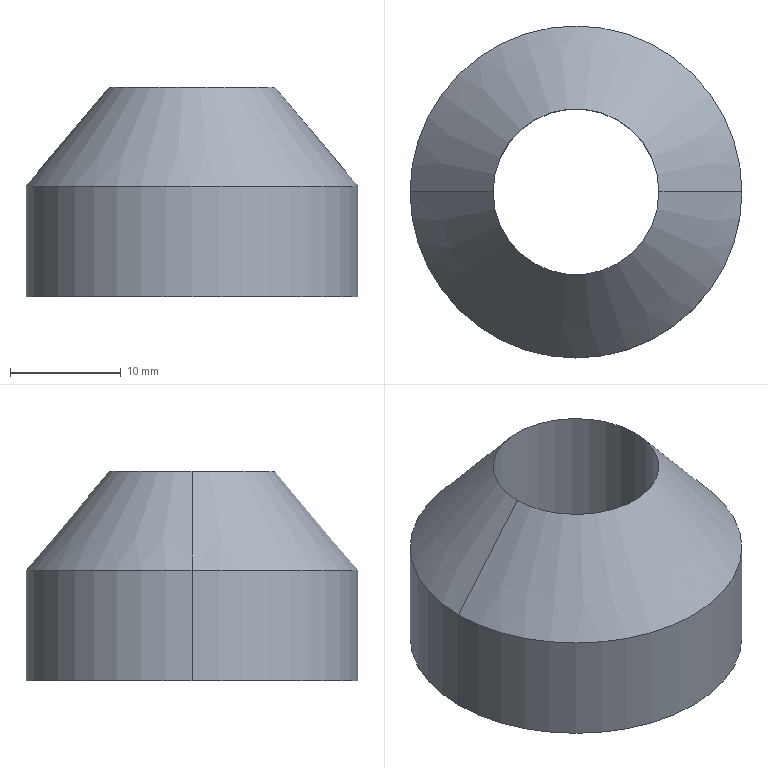Part | SolidWorks | features Chamfer 1, Extrusion 1 | 1 solid | 7 faces | box 30 x 30 x 18.938 mm | volume 7407 mm3 | cylinder 4 | cone 2 | plane 1 | commonest cylinder face diameters 15 x2 30 x2
STEP:
#1=CARTESIAN_POINT('',(7.5,0.,18.938));
#2=VERTEX_POINT('',#1);
#3=CARTESIAN_POINT('',(-7.5,0.,18.938));
#4=VERTEX_POINT('',#3);
#5=CARTESIAN_POINT('',(0.,0.,18.938));
#6=DIRECTION('',(0.,0.,1.));
#7=DIRECTION('',(-1.,0.,0.));
#8=AXIS2_PLACEMENT_3D('',#5,#6,#7);
#9=CIRCLE('',#8,7.5);
#10=EDGE_CURVE('',#2,#4,#9,.T.);
#11=ORIENTED_EDGE('',*,*,#10,.F.);
#12=CARTESIAN_POINT('',(15.,0.,10.));
#13=VERTEX_POINT('',#12);
#14=CARTESIAN_POINT('',(6.609,0.,20.));
#15=DIRECTION('',(0.6428,0.,-0.766));
#16=VECTOR('',#15,1000.);
#17=LINE('',#14,#16);
#18=EDGE_CURVE('',#2,#13,#17,.T.);
#19=ORIENTED_EDGE('',*,*,#18,.T.);
#20=CARTESIAN_POINT('',(-15.,0.,10.));
#21=VERTEX_POINT('',#20);
#22=CARTESIAN_POINT('',(0.,0.,10.));
#23=DIRECTION('',(0.,0.,-1.));
#24=DIRECTION('',(1.,0.,0.));
#25=AXIS2_PLACEMENT_3D('',#22,#23,#24);
#26=CIRCLE('',#25,15.);
#27=EDGE_CURVE('',#21,#13,#26,.T.);
#28=ORIENTED_EDGE('',*,*,#27,.F.);
#29=CARTESIAN_POINT('',(-6.609,0.,20.));
#30=DIRECTION('',(-0.6428,0.,-0.766));
#31=VECTOR('',#30,1000.);
#32=LINE('',#29,#31);
#33=EDGE_CURVE('',#4,#21,#32,.T.);
#34=ORIENTED_EDGE('',*,*,#33,.F.);
#35=EDGE_LOOP('',(#11,#19,#28,#34));
#36=FACE_OUTER_BOUND('',#35,.T.);
#37=CARTESIAN_POINT('',(0.,0.,20.));
#38=DIRECTION('',(0.,0.,-1.));
#39=DIRECTION('',(-1.,0.,0.));
#40=AXIS2_PLACEMENT_3D('',#37,#38,#39);
#41=CONICAL_SURFACE('',#40,6.609,0.6981);
#42=ADVANCED_FACE('',(#36),#41,.T.);
#43=CARTESIAN_POINT('',(0.,0.,18.938));
#44=DIRECTION('',(0.,0.,1.));
#45=DIRECTION('',(-1.,0.,0.));
#46=AXIS2_PLACEMENT_3D('',#43,#44,#45);
#47=CIRCLE('',#46,7.5);
#48=EDGE_CURVE('',#4,#2,#47,.T.);
#49=ORIENTED_EDGE('',*,*,#48,.T.);
#50=CARTESIAN_POINT('',(7.5,0.,0.));
#51=VERTEX_POINT('',#50);
#52=CARTESIAN_POINT('',(7.5,0.,20.));
#53=DIRECTION('',(0.,0.,-1.));
#54=VECTOR('',#53,1000.);
#55=LINE('',#52,#54);
#56=EDGE_CURVE('',#2,#51,#55,.T.);
#57=ORIENTED_EDGE('',*,*,#56,.T.);
#58=CARTESIAN_POINT('',(-7.5,0.,0.));
#59=VERTEX_POINT('',#58);
#60=CARTESIAN_POINT('',(0.,0.,0.));
#61=DIRECTION('',(0.,0.,1.));
#62=DIRECTION('',(1.,0.,0.));
#63=AXIS2_PLACEMENT_3D('',#60,#61,#62);
#64=CIRCLE('',#63,7.5);
#65=EDGE_CURVE('',#59,#51,#64,.T.);
#66=ORIENTED_EDGE('',*,*,#65,.F.);
#67=CARTESIAN_POINT('',(-7.5,0.,20.));
#68=DIRECTION('',(0.,0.,-1.));
#69=VECTOR('',#68,1000.);
#70=LINE('',#67,#69);
#71=EDGE_CURVE('',#4,#59,#70,.T.);
#72=ORIENTED_EDGE('',*,*,#71,.F.);
#73=EDGE_LOOP('',(#49,#57,#66,#72));
#74=FACE_OUTER_BOUND('',#73,.T.);
#75=CARTESIAN_POINT('',(0.,0.,20.));
#76=DIRECTION('',(0.,0.,-1.));
#77=DIRECTION('',(-1.,0.,0.));
#78=AXIS2_PLACEMENT_3D('',#75,#76,#77);
#79=CYLINDRICAL_SURFACE('',#78,7.5);
#80=ADVANCED_FACE('',(#74),#79,.F.);
#81=ORIENTED_EDGE('',*,*,#27,.T.);
#82=CARTESIAN_POINT('',(15.,0.,0.));
#83=VERTEX_POINT('',#82);
#84=CARTESIAN_POINT('',(15.,0.,20.));
#85=DIRECTION('',(0.,0.,-1.));
#86=VECTOR('',#85,1000.);
#87=LINE('',#84,#86);
#88=EDGE_CURVE('',#13,#83,#87,.T.);
#89=ORIENTED_EDGE('',*,*,#88,.T.);
#90=CARTESIAN_POINT('',(-15.,0.,0.));
#91=VERTEX_POINT('',#90);
#92=CARTESIAN_POINT('',(0.,0.,0.));
#93=DIRECTION('',(0.,0.,1.));
#94=DIRECTION('',(1.,0.,0.));
#95=AXIS2_PLACEMENT_3D('',#92,#93,#94);
#96=CIRCLE('',#95,15.);
#97=EDGE_CURVE('',#83,#91,#96,.T.);
#98=ORIENTED_EDGE('',*,*,#97,.T.);
#99=CARTESIAN_POINT('',(-15.,0.,20.));
#100=DIRECTION('',(0.,0.,-1.));
#101=VECTOR('',#100,1000.);
#102=LINE('',#99,#101);
#103=EDGE_CURVE('',#21,#91,#102,.T.);
#104=ORIENTED_EDGE('',*,*,#103,.F.);
#105=EDGE_LOOP('',(#81,#89,#98,#104));
#106=FACE_OUTER_BOUND('',#105,.T.);
#107=CARTESIAN_POINT('',(0.,0.,20.));
#108=DIRECTION('',(0.,0.,-1.));
#109=DIRECTION('',(-1.,0.,0.));
#110=AXIS2_PLACEMENT_3D('',#107,#108,#109);
#111=CYLINDRICAL_SURFACE('',#110,15.);
#112=ADVANCED_FACE('',(#106),#111,.T.);
#113=CARTESIAN_POINT('',(0.,0.,0.));
#114=DIRECTION('',(0.,0.,1.));
#115=DIRECTION('',(1.,0.,0.));
#116=AXIS2_PLACEMENT_3D('',#113,#114,#115);
#117=CIRCLE('',#116,15.);
#118=EDGE_CURVE('',#91,#83,#117,.T.);
#119=ORIENTED_EDGE('',*,*,#118,.F.);
#120=ORIENTED_EDGE('',*,*,#97,.F.);
#121=EDGE_LOOP('',(#119,#120));
#122=FACE_OUTER_BOUND('',#121,.T.);
#123=ORIENTED_EDGE('',*,*,#65,.T.);
#124=CARTESIAN_POINT('',(0.,0.,0.));
#125=DIRECTION('',(0.,0.,1.));
#126=DIRECTION('',(1.,0.,0.));
#127=AXIS2_PLACEMENT_3D('',#124,#125,#126);
#128=CIRCLE('',#127,7.5);
#129=EDGE_CURVE('',#51,#59,#128,.T.);
#130=ORIENTED_EDGE('',*,*,#129,.T.);
#131=EDGE_LOOP('',(#123,#130));
#132=FACE_BOUND('',#131,.T.);
#133=CARTESIAN_POINT('',(0.,0.,0.));
#134=DIRECTION('',(0.,0.,1.));
#135=DIRECTION('',(1.,0.,0.));
#136=AXIS2_PLACEMENT_3D('',#133,#134,#135);
#137=PLANE('',#136);
#138=ADVANCED_FACE('',(#122,#132),#137,.F.);
#139=ORIENTED_EDGE('',*,*,#88,.F.);
#140=CARTESIAN_POINT('',(0.,0.,10.));
#141=DIRECTION('',(0.,0.,-1.));
#142=DIRECTION('',(1.,0.,0.));
#143=AXIS2_PLACEMENT_3D('',#140,#141,#142);
#144=CIRCLE('',#143,15.);
#145=EDGE_CURVE('',#13,#21,#144,.T.);
#146=ORIENTED_EDGE('',*,*,#145,.T.);
#147=ORIENTED_EDGE('',*,*,#103,.T.);
#148=ORIENTED_EDGE('',*,*,#118,.T.);
#149=EDGE_LOOP('',(#139,#146,#147,#148));
#150=FACE_OUTER_BOUND('',#149,.T.);
#151=CARTESIAN_POINT('',(0.,0.,20.));
#152=DIRECTION('',(0.,0.,-1.));
#153=DIRECTION('',(-1.,0.,0.));
#154=AXIS2_PLACEMENT_3D('',#151,#152,#153);
#155=CYLINDRICAL_SURFACE('',#154,15.);
#156=ADVANCED_FACE('',(#150),#155,.T.);
#157=ORIENTED_EDGE('',*,*,#56,.F.);
#158=ORIENTED_EDGE('',*,*,#10,.T.);
#159=ORIENTED_EDGE('',*,*,#71,.T.);
#160=ORIENTED_EDGE('',*,*,#129,.F.);
#161=EDGE_LOOP('',(#157,#158,#159,#160));
#162=FACE_OUTER_BOUND('',#161,.T.);
#163=CARTESIAN_POINT('',(0.,0.,20.));
#164=DIRECTION('',(0.,0.,-1.));
#165=DIRECTION('',(-1.,0.,0.));
#166=AXIS2_PLACEMENT_3D('',#163,#164,#165);
#167=CYLINDRICAL_SURFACE('',#166,7.5);
#168=ADVANCED_FACE('',(#162),#167,.F.);
#169=ORIENTED_EDGE('',*,*,#18,.F.);
#170=ORIENTED_EDGE('',*,*,#48,.F.);
#171=ORIENTED_EDGE('',*,*,#33,.T.);
#172=ORIENTED_EDGE('',*,*,#145,.F.);
#173=EDGE_LOOP('',(#169,#170,#171,#172));
#174=FACE_OUTER_BOUND('',#173,.T.);
#175=CARTESIAN_POINT('',(0.,0.,20.));
#176=DIRECTION('',(0.,0.,-1.));
#177=DIRECTION('',(-1.,0.,0.));
#178=AXIS2_PLACEMENT_3D('',#175,#176,#177);
#179=CONICAL_SURFACE('',#178,6.609,0.6981);
#180=ADVANCED_FACE('',(#174),#179,.T.);
#181=CLOSED_SHELL('',(#42,#80,#112,#138,#156,#168,#180));
#182=MANIFOLD_SOLID_BREP('',#181);
#183=CARTESIAN_POINT('',(0.,0.,0.));
#184=DIRECTION('',(0.,0.,1.));
#185=DIRECTION('',(1.,0.,0.));
#186=AXIS2_PLACEMENT_3D('',#183,#184,#185);
#187=(LENGTH_UNIT()NAMED_UNIT(*)SI_UNIT(.MILLI.,.METRE.));
#188=UNCERTAINTY_MEASURE_WITH_UNIT(LENGTH_MEASURE(0.00001),#187,'','');
#189=(NAMED_UNIT(*)PLANE_ANGLE_UNIT()SI_UNIT($,.RADIAN.));
#190=(NAMED_UNIT(*)SI_UNIT($,.STERADIAN.)SOLID_ANGLE_UNIT());
#191=(GEOMETRIC_REPRESENTATION_CONTEXT(3)GLOBAL_UNCERTAINTY_ASSIGNED_CONTEXT((#188))GLOBAL_UNIT_ASSIGNED_CONTEXT((#187,#189,#190))REPRESENTATION_CONTEXT('',''));
#192=ADVANCED_BREP_SHAPE_REPRESENTATION('',(#182,#186),#191);